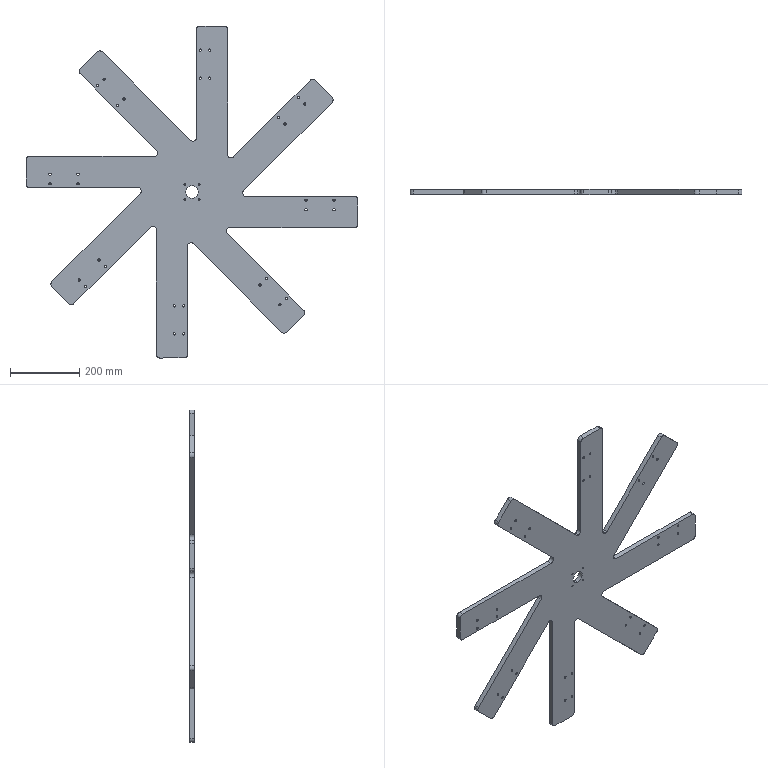Part | SolidWorks | features ICE 7, CirPattern 3, Fillet 3, Extrusion 1 | 1 solid | 128 faces | box 960 x 14 x 960 mm | volume 4425527 mm3 | cylinder 102 | plane 26 | commonest cylinder face diameters 6.6 x64 20 x28 4.4 x8 36 x2